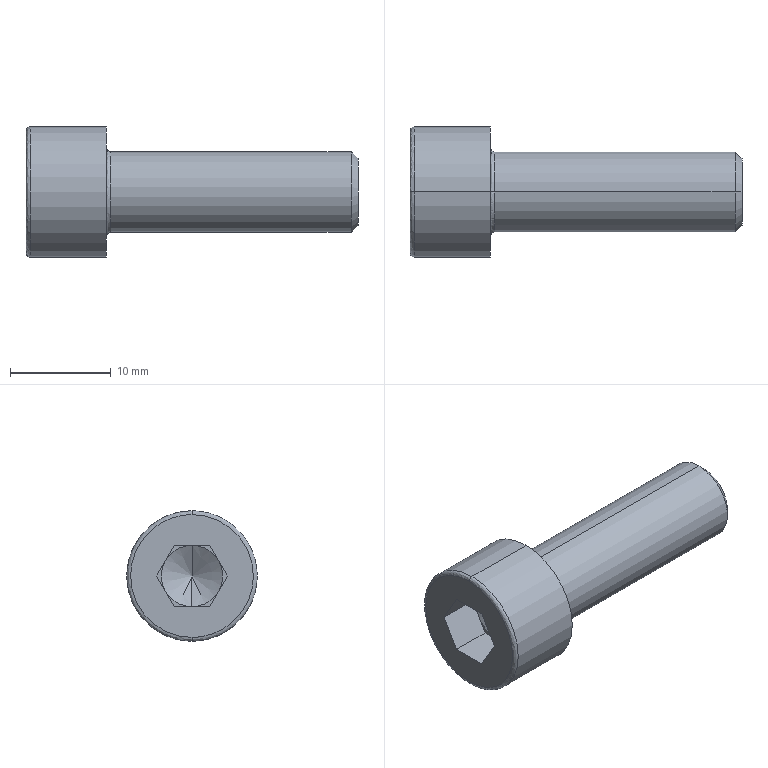Part | STEP file | 0229_310_M8x25 | 1 solid | 27 faces | box 33 x 13 x 13 mm | volume 2167 mm3 | plane 15 | spline 4 | cylinder 4 | cone 4 | commonest cylinder face diameters 8 x2 13 x2